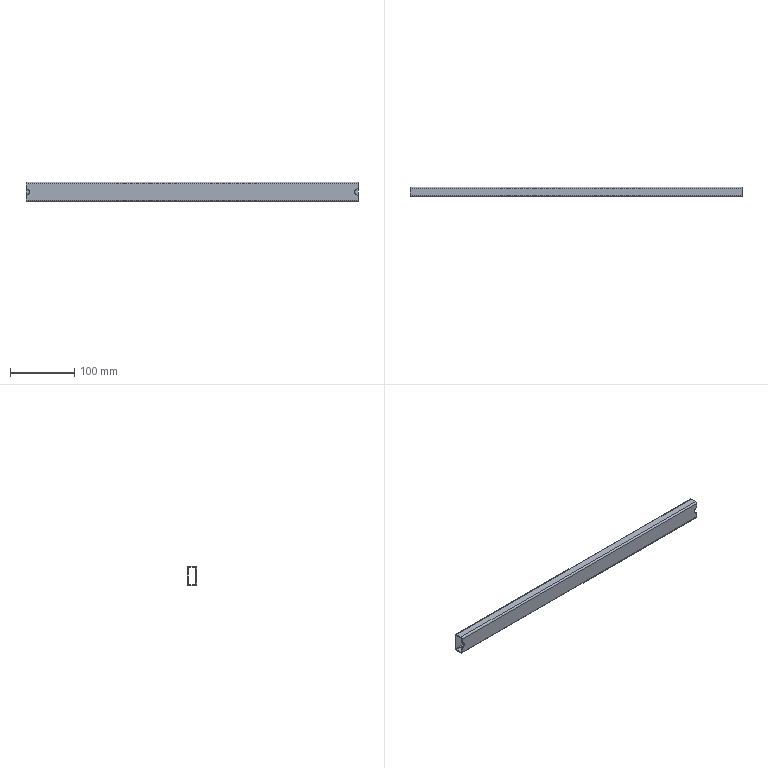Part | STEP file | 6150504 | 1 solid | 20 faces | box 515 x 15 x 30 mm | volume 62451 mm3 | plane 10 | cylinder 10 | commonest cylinder face diameters 2 x4 5 x4 10 x2
STEP:
#1=CARTESIAN_POINT('',(257.5,-7.5,-5.));
#2=VERTEX_POINT('',#1);
#3=CARTESIAN_POINT('',(257.5,-7.5,5.));
#4=VERTEX_POINT('',#3);
#5=CARTESIAN_POINT('',(257.5,-7.5,0.));
#6=DIRECTION('',(0.,1.,0.));
#7=DIRECTION('',(1.,0.,0.));
#8=AXIS2_PLACEMENT_3D('',#5,#6,#7);
#9=CIRCLE('',#8,5.);
#10=EDGE_CURVE('',#2,#4,#9,.T.);
#11=ORIENTED_EDGE('',*,*,#10,.T.);
#12=CARTESIAN_POINT('',(257.5,-7.5,12.5));
#13=VERTEX_POINT('',#12);
#14=CARTESIAN_POINT('',(257.5,-7.5,15.));
#15=DIRECTION('',(0.,0.,-1.));
#16=VECTOR('',#15,1000.);
#17=LINE('',#14,#16);
#18=EDGE_CURVE('',#13,#4,#17,.T.);
#19=ORIENTED_EDGE('',*,*,#18,.F.);
#20=CARTESIAN_POINT('',(-257.5,-7.5,12.5));
#21=VERTEX_POINT('',#20);
#22=CARTESIAN_POINT('',(-257.5,-7.5,12.5));
#23=DIRECTION('',(-1.,0.,0.));
#24=VECTOR('',#23,1000.);
#25=LINE('',#22,#24);
#26=EDGE_CURVE('',#13,#21,#25,.T.);
#27=ORIENTED_EDGE('',*,*,#26,.T.);
#28=CARTESIAN_POINT('',(-257.5,-7.5,5.));
#29=VERTEX_POINT('',#28);
#30=CARTESIAN_POINT('',(-257.5,-7.5,15.));
#31=DIRECTION('',(0.,0.,-1.));
#32=VECTOR('',#31,1000.);
#33=LINE('',#30,#32);
#34=EDGE_CURVE('',#21,#29,#33,.T.);
#35=ORIENTED_EDGE('',*,*,#34,.T.);
#36=CARTESIAN_POINT('',(-257.5,-7.5,-5.));
#37=VERTEX_POINT('',#36);
#38=CARTESIAN_POINT('',(-257.5,-7.5,0.));
#39=DIRECTION('',(0.,1.,0.));
#40=DIRECTION('',(-1.,0.,0.));
#41=AXIS2_PLACEMENT_3D('',#38,#39,#40);
#42=CIRCLE('',#41,5.);
#43=EDGE_CURVE('',#29,#37,#42,.T.);
#44=ORIENTED_EDGE('',*,*,#43,.T.);
#45=CARTESIAN_POINT('',(-257.5,-7.5,-12.5));
#46=VERTEX_POINT('',#45);
#47=CARTESIAN_POINT('',(-257.5,-7.5,15.));
#48=DIRECTION('',(0.,0.,-1.));
#49=VECTOR('',#48,1000.);
#50=LINE('',#47,#49);
#51=EDGE_CURVE('',#37,#46,#50,.T.);
#52=ORIENTED_EDGE('',*,*,#51,.T.);
#53=CARTESIAN_POINT('',(257.5,-7.5,-12.5));
#54=VERTEX_POINT('',#53);
#55=CARTESIAN_POINT('',(-257.5,-7.5,-12.5));
#56=DIRECTION('',(1.,0.,0.));
#57=VECTOR('',#56,1000.);
#58=LINE('',#55,#57);
#59=EDGE_CURVE('',#46,#54,#58,.T.);
#60=ORIENTED_EDGE('',*,*,#59,.T.);
#61=CARTESIAN_POINT('',(257.5,-7.5,15.));
#62=DIRECTION('',(0.,0.,-1.));
#63=VECTOR('',#62,1000.);
#64=LINE('',#61,#63);
#65=EDGE_CURVE('',#2,#54,#64,.T.);
#66=ORIENTED_EDGE('',*,*,#65,.F.);
#67=EDGE_LOOP('',(#11,#19,#27,#35,#44,#52,#60,#66));
#68=FACE_OUTER_BOUND('',#67,.T.);
#69=CARTESIAN_POINT('',(-257.5,-7.5,15.));
#70=DIRECTION('',(0.,1.,0.));
#71=DIRECTION('',(-1.,0.,0.));
#72=AXIS2_PLACEMENT_3D('',#69,#70,#71);
#73=PLANE('',#72);
#74=ADVANCED_FACE('',(#68),#73,.F.);
#75=CARTESIAN_POINT('',(257.5,-6.,12.5));
#76=VERTEX_POINT('',#75);
#77=CARTESIAN_POINT('',(257.5,-6.,5.));
#78=VERTEX_POINT('',#77);
#79=CARTESIAN_POINT('',(257.5,-6.,15.));
#80=DIRECTION('',(0.,0.,-1.));
#81=VECTOR('',#80,1000.);
#82=LINE('',#79,#81);
#83=EDGE_CURVE('',#76,#78,#82,.T.);
#84=ORIENTED_EDGE('',*,*,#83,.T.);
#85=CARTESIAN_POINT('',(257.5,-6.,-5.));
#86=VERTEX_POINT('',#85);
#87=CARTESIAN_POINT('',(257.5,-6.,0.));
#88=DIRECTION('',(0.,-1.,0.));
#89=DIRECTION('',(-1.,0.,0.));
#90=AXIS2_PLACEMENT_3D('',#87,#88,#89);
#91=CIRCLE('',#90,5.);
#92=EDGE_CURVE('',#78,#86,#91,.T.);
#93=ORIENTED_EDGE('',*,*,#92,.T.);
#94=CARTESIAN_POINT('',(257.5,-6.,-12.5));
#95=VERTEX_POINT('',#94);
#96=CARTESIAN_POINT('',(257.5,-6.,15.));
#97=DIRECTION('',(0.,0.,-1.));
#98=VECTOR('',#97,1000.);
#99=LINE('',#96,#98);
#100=EDGE_CURVE('',#86,#95,#99,.T.);
#101=ORIENTED_EDGE('',*,*,#100,.T.);
#102=CARTESIAN_POINT('',(-257.5,-6.,-12.5));
#103=VERTEX_POINT('',#102);
#104=CARTESIAN_POINT('',(-257.5,-6.,-12.5));
#105=DIRECTION('',(1.,0.,0.));
#106=VECTOR('',#105,1000.);
#107=LINE('',#104,#106);
#108=EDGE_CURVE('',#103,#95,#107,.T.);
#109=ORIENTED_EDGE('',*,*,#108,.F.);
#110=CARTESIAN_POINT('',(-257.5,-6.,-5.));
#111=VERTEX_POINT('',#110);
#112=CARTESIAN_POINT('',(-257.5,-6.,15.));
#113=DIRECTION('',(0.,0.,-1.));
#114=VECTOR('',#113,1000.);
#115=LINE('',#112,#114);
#116=EDGE_CURVE('',#111,#103,#115,.T.);
#117=ORIENTED_EDGE('',*,*,#116,.F.);
#118=CARTESIAN_POINT('',(-257.5,-6.,5.));
#119=VERTEX_POINT('',#118);
#120=CARTESIAN_POINT('',(-257.5,-6.,0.));
#121=DIRECTION('',(0.,-1.,0.));
#122=DIRECTION('',(-1.,0.,0.));
#123=AXIS2_PLACEMENT_3D('',#120,#121,#122);
#124=CIRCLE('',#123,5.);
#125=EDGE_CURVE('',#111,#119,#124,.T.);
#126=ORIENTED_EDGE('',*,*,#125,.T.);
#127=CARTESIAN_POINT('',(-257.5,-6.,12.5));
#128=VERTEX_POINT('',#127);
#129=CARTESIAN_POINT('',(-257.5,-6.,15.));
#130=DIRECTION('',(0.,0.,-1.));
#131=VECTOR('',#130,1000.);
#132=LINE('',#129,#131);
#133=EDGE_CURVE('',#128,#119,#132,.T.);
#134=ORIENTED_EDGE('',*,*,#133,.F.);
#135=CARTESIAN_POINT('',(-257.5,-6.,12.5));
#136=DIRECTION('',(-1.,0.,0.));
#137=VECTOR('',#136,1000.);
#138=LINE('',#135,#137);
#139=EDGE_CURVE('',#76,#128,#138,.T.);
#140=ORIENTED_EDGE('',*,*,#139,.F.);
#141=EDGE_LOOP('',(#84,#93,#101,#109,#117,#126,#134,#140));
#142=FACE_OUTER_BOUND('',#141,.T.);
#143=CARTESIAN_POINT('',(-257.5,-6.,15.));
#144=DIRECTION('',(0.,1.,0.));
#145=DIRECTION('',(-1.,0.,0.));
#146=AXIS2_PLACEMENT_3D('',#143,#144,#145);
#147=PLANE('',#146);
#148=ADVANCED_FACE('',(#142),#147,.T.);
#149=CARTESIAN_POINT('',(257.5,-3.,-5.));
#150=DIRECTION('',(0.,1.,0.));
#151=VECTOR('',#150,1000.);
#152=LINE('',#149,#151);
#153=EDGE_CURVE('',#2,#86,#152,.T.);
#154=ORIENTED_EDGE('',*,*,#153,.F.);
#155=ORIENTED_EDGE('',*,*,#65,.T.);
#156=CARTESIAN_POINT('',(257.5,-5.,-15.));
#157=VERTEX_POINT('',#156);
#158=CARTESIAN_POINT('',(257.5,-5.,-12.5));
#159=DIRECTION('',(1.,0.,0.));
#160=DIRECTION('',(0.,0.,1.));
#161=AXIS2_PLACEMENT_3D('',#158,#159,#160);
#162=CIRCLE('',#161,2.5);
#163=EDGE_CURVE('',#54,#157,#162,.T.);
#164=ORIENTED_EDGE('',*,*,#163,.T.);
#165=CARTESIAN_POINT('',(257.5,5.,-15.));
#166=VERTEX_POINT('',#165);
#167=CARTESIAN_POINT('',(257.5,7.5,-15.));
#168=DIRECTION('',(0.,1.,0.));
#169=VECTOR('',#168,1000.);
#170=LINE('',#167,#169);
#171=EDGE_CURVE('',#157,#166,#170,.T.);
#172=ORIENTED_EDGE('',*,*,#171,.T.);
#173=CARTESIAN_POINT('',(257.5,7.5,-12.5));
#174=VERTEX_POINT('',#173);
#175=CARTESIAN_POINT('',(257.5,5.,-12.5));
#176=DIRECTION('',(1.,0.,0.));
#177=DIRECTION('',(0.,0.,1.));
#178=AXIS2_PLACEMENT_3D('',#175,#176,#177);
#179=CIRCLE('',#178,2.5);
#180=EDGE_CURVE('',#166,#174,#179,.T.);
#181=ORIENTED_EDGE('',*,*,#180,.T.);
#182=CARTESIAN_POINT('',(257.5,7.5,12.5));
#183=VERTEX_POINT('',#182);
#184=CARTESIAN_POINT('',(257.5,7.5,15.));
#185=DIRECTION('',(0.,0.,-1.));
#186=VECTOR('',#185,1000.);
#187=LINE('',#184,#186);
#188=EDGE_CURVE('',#183,#174,#187,.T.);
#189=ORIENTED_EDGE('',*,*,#188,.F.);
#190=CARTESIAN_POINT('',(257.5,5.,15.));
#191=VERTEX_POINT('',#190);
#192=CARTESIAN_POINT('',(257.5,5.,12.5));
#193=DIRECTION('',(1.,0.,0.));
#194=DIRECTION('',(0.,0.,1.));
#195=AXIS2_PLACEMENT_3D('',#192,#193,#194);
#196=CIRCLE('',#195,2.5);
#197=EDGE_CURVE('',#183,#191,#196,.T.);
#198=ORIENTED_EDGE('',*,*,#197,.T.);
#199=CARTESIAN_POINT('',(257.5,-5.,15.));
#200=VERTEX_POINT('',#199);
#201=CARTESIAN_POINT('',(257.5,7.5,15.));
#202=DIRECTION('',(0.,1.,0.));
#203=VECTOR('',#202,1000.);
#204=LINE('',#201,#203);
#205=EDGE_CURVE('',#200,#191,#204,.T.);
#206=ORIENTED_EDGE('',*,*,#205,.F.);
#207=CARTESIAN_POINT('',(257.5,-5.,12.5));
#208=DIRECTION('',(1.,0.,0.));
#209=DIRECTION('',(0.,0.,1.));
#210=AXIS2_PLACEMENT_3D('',#207,#208,#209);
#211=CIRCLE('',#210,2.5);
#212=EDGE_CURVE('',#200,#13,#211,.T.);
#213=ORIENTED_EDGE('',*,*,#212,.T.);
#214=ORIENTED_EDGE('',*,*,#18,.T.);
#215=CARTESIAN_POINT('',(257.5,-3.,5.));
#216=DIRECTION('',(0.,-1.,0.));
#217=VECTOR('',#216,1000.);
#218=LINE('',#215,#217);
#219=EDGE_CURVE('',#78,#4,#218,.T.);
#220=ORIENTED_EDGE('',*,*,#219,.F.);
#221=ORIENTED_EDGE('',*,*,#83,.F.);
#222=CARTESIAN_POINT('',(257.5,-5.,13.5));
#223=VERTEX_POINT('',#222);
#224=CARTESIAN_POINT('',(257.5,-5.,12.5));
#225=DIRECTION('',(1.,0.,0.));
#226=DIRECTION('',(0.,0.,1.));
#227=AXIS2_PLACEMENT_3D('',#224,#225,#226);
#228=CIRCLE('',#227,1.);
#229=EDGE_CURVE('',#223,#76,#228,.T.);
#230=ORIENTED_EDGE('',*,*,#229,.F.);
#231=CARTESIAN_POINT('',(257.5,5.,13.5));
#232=VERTEX_POINT('',#231);
#233=CARTESIAN_POINT('',(257.5,7.5,13.5));
#234=DIRECTION('',(0.,1.,0.));
#235=VECTOR('',#234,1000.);
#236=LINE('',#233,#235);
#237=EDGE_CURVE('',#223,#232,#236,.T.);
#238=ORIENTED_EDGE('',*,*,#237,.T.);
#239=CARTESIAN_POINT('',(257.5,6.,12.5));
#240=VERTEX_POINT('',#239);
#241=CARTESIAN_POINT('',(257.5,5.,12.5));
#242=DIRECTION('',(1.,0.,0.));
#243=DIRECTION('',(0.,0.,1.));
#244=AXIS2_PLACEMENT_3D('',#241,#242,#243);
#245=CIRCLE('',#244,1.);
#246=EDGE_CURVE('',#240,#232,#245,.T.);
#247=ORIENTED_EDGE('',*,*,#246,.F.);
#248=CARTESIAN_POINT('',(257.5,6.,-12.5));
#249=VERTEX_POINT('',#248);
#250=CARTESIAN_POINT('',(257.5,6.,15.));
#251=DIRECTION('',(0.,0.,-1.));
#252=VECTOR('',#251,1000.);
#253=LINE('',#250,#252);
#254=EDGE_CURVE('',#240,#249,#253,.T.);
#255=ORIENTED_EDGE('',*,*,#254,.T.);
#256=CARTESIAN_POINT('',(257.5,5.,-13.5));
#257=VERTEX_POINT('',#256);
#258=CARTESIAN_POINT('',(257.5,5.,-12.5));
#259=DIRECTION('',(1.,0.,0.));
#260=DIRECTION('',(0.,0.,1.));
#261=AXIS2_PLACEMENT_3D('',#258,#259,#260);
#262=CIRCLE('',#261,1.);
#263=EDGE_CURVE('',#257,#249,#262,.T.);
#264=ORIENTED_EDGE('',*,*,#263,.F.);
#265=CARTESIAN_POINT('',(257.5,-5.,-13.5));
#266=VERTEX_POINT('',#265);
#267=CARTESIAN_POINT('',(257.5,7.5,-13.5));
#268=DIRECTION('',(0.,1.,0.));
#269=VECTOR('',#268,1000.);
#270=LINE('',#267,#269);
#271=EDGE_CURVE('',#266,#257,#270,.T.);
#272=ORIENTED_EDGE('',*,*,#271,.F.);
#273=CARTESIAN_POINT('',(257.5,-5.,-12.5));
#274=DIRECTION('',(1.,0.,0.));
#275=DIRECTION('',(0.,0.,1.));
#276=AXIS2_PLACEMENT_3D('',#273,#274,#275);
#277=CIRCLE('',#276,1.);
#278=EDGE_CURVE('',#95,#266,#277,.T.);
#279=ORIENTED_EDGE('',*,*,#278,.F.);
#280=ORIENTED_EDGE('',*,*,#100,.F.);
#281=EDGE_LOOP('',(#154,#155,#164,#172,#181,#189,#198,#206,#213,#214,#220,#221,#230,#238,#247,#255,#264,#272,#279,#280));
#282=FACE_OUTER_BOUND('',#281,.T.);
#283=CARTESIAN_POINT('',(257.5,7.5,15.));
#284=DIRECTION('',(-1.,0.,0.));
#285=DIRECTION('',(0.,0.,1.));
#286=AXIS2_PLACEMENT_3D('',#283,#284,#285);
#287=PLANE('',#286);
#288=ADVANCED_FACE('',(#282),#287,.F.);
#289=CARTESIAN_POINT('',(-257.5,-3.,5.));
#290=DIRECTION('',(0.,1.,0.));
#291=VECTOR('',#290,1000.);
#292=LINE('',#289,#291);
#293=EDGE_CURVE('',#29,#119,#292,.T.);
#294=ORIENTED_EDGE('',*,*,#293,.F.);
#295=ORIENTED_EDGE('',*,*,#34,.F.);
#296=CARTESIAN_POINT('',(-257.5,-5.,15.));
#297=VERTEX_POINT('',#296);
#298=CARTESIAN_POINT('',(-257.5,-5.,12.5));
#299=DIRECTION('',(-1.,0.,0.));
#300=DIRECTION('',(0.,0.,-1.));
#301=AXIS2_PLACEMENT_3D('',#298,#299,#300);
#302=CIRCLE('',#301,2.5);
#303=EDGE_CURVE('',#21,#297,#302,.T.);
#304=ORIENTED_EDGE('',*,*,#303,.T.);
#305=CARTESIAN_POINT('',(-257.5,5.,15.));
#306=VERTEX_POINT('',#305);
#307=CARTESIAN_POINT('',(-257.5,7.5,15.));
#308=DIRECTION('',(0.,-1.,0.));
#309=VECTOR('',#308,1000.);
#310=LINE('',#307,#309);
#311=EDGE_CURVE('',#306,#297,#310,.T.);
#312=ORIENTED_EDGE('',*,*,#311,.F.);
#313=CARTESIAN_POINT('',(-257.5,7.5,12.5));
#314=VERTEX_POINT('',#313);
#315=CARTESIAN_POINT('',(-257.5,5.,12.5));
#316=DIRECTION('',(-1.,0.,0.));
#317=DIRECTION('',(0.,0.,-1.));
#318=AXIS2_PLACEMENT_3D('',#315,#316,#317);
#319=CIRCLE('',#318,2.5);
#320=EDGE_CURVE('',#306,#314,#319,.T.);
#321=ORIENTED_EDGE('',*,*,#320,.T.);
#322=CARTESIAN_POINT('',(-257.5,7.5,-12.5));
#323=VERTEX_POINT('',#322);
#324=CARTESIAN_POINT('',(-257.5,7.5,15.));
#325=DIRECTION('',(0.,0.,-1.));
#326=VECTOR('',#325,1000.);
#327=LINE('',#324,#326);
#328=EDGE_CURVE('',#314,#323,#327,.T.);
#329=ORIENTED_EDGE('',*,*,#328,.T.);
#330=CARTESIAN_POINT('',(-257.5,5.,-15.));
#331=VERTEX_POINT('',#330);
#332=CARTESIAN_POINT('',(-257.5,5.,-12.5));
#333=DIRECTION('',(-1.,0.,0.));
#334=DIRECTION('',(0.,0.,-1.));
#335=AXIS2_PLACEMENT_3D('',#332,#333,#334);
#336=CIRCLE('',#335,2.5);
#337=EDGE_CURVE('',#323,#331,#336,.T.);
#338=ORIENTED_EDGE('',*,*,#337,.T.);
#339=CARTESIAN_POINT('',(-257.5,-5.,-15.));
#340=VERTEX_POINT('',#339);
#341=CARTESIAN_POINT('',(-257.5,7.5,-15.));
#342=DIRECTION('',(0.,-1.,0.));
#343=VECTOR('',#342,1000.);
#344=LINE('',#341,#343);
#345=EDGE_CURVE('',#331,#340,#344,.T.);
#346=ORIENTED_EDGE('',*,*,#345,.T.);
#347=CARTESIAN_POINT('',(-257.5,-5.,-12.5));
#348=DIRECTION('',(-1.,0.,0.));
#349=DIRECTION('',(0.,0.,-1.));
#350=AXIS2_PLACEMENT_3D('',#347,#348,#349);
#351=CIRCLE('',#350,2.5);
#352=EDGE_CURVE('',#340,#46,#351,.T.);
#353=ORIENTED_EDGE('',*,*,#352,.T.);
#354=ORIENTED_EDGE('',*,*,#51,.F.);
#355=CARTESIAN_POINT('',(-257.5,-3.,-5.));
#356=DIRECTION('',(0.,-1.,0.));
#357=VECTOR('',#356,1000.);
#358=LINE('',#355,#357);
#359=EDGE_CURVE('',#111,#37,#358,.T.);
#360=ORIENTED_EDGE('',*,*,#359,.F.);
#361=ORIENTED_EDGE('',*,*,#116,.T.);
#362=CARTESIAN_POINT('',(-257.5,-5.,-13.5));
#363=VERTEX_POINT('',#362);
#364=CARTESIAN_POINT('',(-257.5,-5.,-12.5));
#365=DIRECTION('',(-1.,0.,0.));
#366=DIRECTION('',(0.,0.,-1.));
#367=AXIS2_PLACEMENT_3D('',#364,#365,#366);
#368=CIRCLE('',#367,1.);
#369=EDGE_CURVE('',#363,#103,#368,.T.);
#370=ORIENTED_EDGE('',*,*,#369,.F.);
#371=CARTESIAN_POINT('',(-257.5,5.,-13.5));
#372=VERTEX_POINT('',#371);
#373=CARTESIAN_POINT('',(-257.5,7.5,-13.5));
#374=DIRECTION('',(0.,-1.,0.));
#375=VECTOR('',#374,1000.);
#376=LINE('',#373,#375);
#377=EDGE_CURVE('',#372,#363,#376,.T.);
#378=ORIENTED_EDGE('',*,*,#377,.F.);
#379=CARTESIAN_POINT('',(-257.5,6.,-12.5));
#380=VERTEX_POINT('',#379);
#381=CARTESIAN_POINT('',(-257.5,5.,-12.5));
#382=DIRECTION('',(-1.,0.,0.));
#383=DIRECTION('',(0.,0.,-1.));
#384=AXIS2_PLACEMENT_3D('',#381,#382,#383);
#385=CIRCLE('',#384,1.);
#386=EDGE_CURVE('',#380,#372,#385,.T.);
#387=ORIENTED_EDGE('',*,*,#386,.F.);
#388=CARTESIAN_POINT('',(-257.5,6.,12.5));
#389=VERTEX_POINT('',#388);
#390=CARTESIAN_POINT('',(-257.5,6.,15.));
#391=DIRECTION('',(0.,0.,-1.));
#392=VECTOR('',#391,1000.);
#393=LINE('',#390,#392);
#394=EDGE_CURVE('',#389,#380,#393,.T.);
#395=ORIENTED_EDGE('',*,*,#394,.F.);
#396=CARTESIAN_POINT('',(-257.5,5.,13.5));
#397=VERTEX_POINT('',#396);
#398=CARTESIAN_POINT('',(-257.5,5.,12.5));
#399=DIRECTION('',(-1.,0.,0.));
#400=DIRECTION('',(0.,0.,-1.));
#401=AXIS2_PLACEMENT_3D('',#398,#399,#400);
#402=CIRCLE('',#401,1.);
#403=EDGE_CURVE('',#397,#389,#402,.T.);
#404=ORIENTED_EDGE('',*,*,#403,.F.);
#405=CARTESIAN_POINT('',(-257.5,-5.,13.5));
#406=VERTEX_POINT('',#405);
#407=CARTESIAN_POINT('',(-257.5,7.5,13.5));
#408=DIRECTION('',(0.,-1.,0.));
#409=VECTOR('',#408,1000.);
#410=LINE('',#407,#409);
#411=EDGE_CURVE('',#397,#406,#410,.T.);
#412=ORIENTED_EDGE('',*,*,#411,.T.);
#413=CARTESIAN_POINT('',(-257.5,-5.,12.5));
#414=DIRECTION('',(-1.,0.,0.));
#415=DIRECTION('',(0.,0.,-1.));
#416=AXIS2_PLACEMENT_3D('',#413,#414,#415);
#417=CIRCLE('',#416,1.);
#418=EDGE_CURVE('',#128,#406,#417,.T.);
#419=ORIENTED_EDGE('',*,*,#418,.F.);
#420=ORIENTED_EDGE('',*,*,#133,.T.);
#421=EDGE_LOOP('',(#294,#295,#304,#312,#321,#329,#338,#346,#353,#354,#360,#361,#370,#378,#387,#395,#404,#412,#419,#420));
#422=FACE_OUTER_BOUND('',#421,.T.);
#423=CARTESIAN_POINT('',(-257.5,7.5,15.));
#424=DIRECTION('',(1.,0.,0.));
#425=DIRECTION('',(0.,0.,-1.));
#426=AXIS2_PLACEMENT_3D('',#423,#424,#425);
#427=PLANE('',#426);
#428=ADVANCED_FACE('',(#422),#427,.F.);
#429=ORIENTED_EDGE('',*,*,#188,.T.);
#430=CARTESIAN_POINT('',(-257.5,7.5,-12.5));
#431=DIRECTION('',(-1.,0.,0.));
#432=VECTOR('',#431,1000.);
#433=LINE('',#430,#432);
#434=EDGE_CURVE('',#174,#323,#433,.T.);
#435=ORIENTED_EDGE('',*,*,#434,.T.);
#436=ORIENTED_EDGE('',*,*,#328,.F.);
#437=CARTESIAN_POINT('',(257.5,7.5,12.5));
#438=DIRECTION('',(1.,0.,0.));
#439=VECTOR('',#438,1000.);
#440=LINE('',#437,#439);
#441=EDGE_CURVE('',#314,#183,#440,.T.);
#442=ORIENTED_EDGE('',*,*,#441,.T.);
#443=EDGE_LOOP('',(#429,#435,#436,#442));
#444=FACE_OUTER_BOUND('',#443,.T.);
#445=CARTESIAN_POINT('',(-257.5,7.5,15.));
#446=DIRECTION('',(0.,-1.,0.));
#447=DIRECTION('',(0.,0.,-1.));
#448=AXIS2_PLACEMENT_3D('',#445,#446,#447);
#449=PLANE('',#448);
#450=ADVANCED_FACE('',(#444),#449,.F.);
#451=ORIENTED_EDGE('',*,*,#311,.T.);
#452=CARTESIAN_POINT('',(257.5,-5.,15.));
#453=DIRECTION('',(1.,0.,0.));
#454=VECTOR('',#453,1000.);
#455=LINE('',#452,#454);
#456=EDGE_CURVE('',#297,#200,#455,.T.);
#457=ORIENTED_EDGE('',*,*,#456,.T.);
#458=ORIENTED_EDGE('',*,*,#205,.T.);
#459=CARTESIAN_POINT('',(-257.5,5.,15.));
#460=DIRECTION('',(-1.,0.,0.));
#461=VECTOR('',#460,1000.);
#462=LINE('',#459,#461);
#463=EDGE_CURVE('',#191,#306,#462,.T.);
#464=ORIENTED_EDGE('',*,*,#463,.T.);
#465=EDGE_LOOP('',(#451,#457,#458,#464));
#466=FACE_OUTER_BOUND('',#465,.T.);
#467=CARTESIAN_POINT('',(-257.5,7.5,15.));
#468=DIRECTION('',(0.,0.,1.));
#469=DIRECTION('',(1.,0.,0.));
#470=AXIS2_PLACEMENT_3D('',#467,#468,#469);
#471=PLANE('',#470);
#472=ADVANCED_FACE('',(#466),#471,.T.);
#473=ORIENTED_EDGE('',*,*,#345,.F.);
#474=CARTESIAN_POINT('',(-257.5,5.,-15.));
#475=DIRECTION('',(1.,0.,0.));
#476=VECTOR('',#475,1000.);
#477=LINE('',#474,#476);
#478=EDGE_CURVE('',#331,#166,#477,.T.);
#479=ORIENTED_EDGE('',*,*,#478,.T.);
#480=ORIENTED_EDGE('',*,*,#171,.F.);
#481=CARTESIAN_POINT('',(-257.5,-5.,-15.));
#482=DIRECTION('',(-1.,0.,0.));
#483=VECTOR('',#482,1000.);
#484=LINE('',#481,#483);
#485=EDGE_CURVE('',#157,#340,#484,.T.);
#486=ORIENTED_EDGE('',*,*,#485,.T.);
#487=EDGE_LOOP('',(#473,#479,#480,#486));
#488=FACE_OUTER_BOUND('',#487,.T.);
#489=CARTESIAN_POINT('',(-257.5,7.5,-15.));
#490=DIRECTION('',(0.,0.,1.));
#491=DIRECTION('',(1.,0.,0.));
#492=AXIS2_PLACEMENT_3D('',#489,#490,#491);
#493=PLANE('',#492);
#494=ADVANCED_FACE('',(#488),#493,.F.);
#495=ORIENTED_EDGE('',*,*,#303,.F.);
#496=ORIENTED_EDGE('',*,*,#26,.F.);
#497=ORIENTED_EDGE('',*,*,#212,.F.);
#498=ORIENTED_EDGE('',*,*,#456,.F.);
#499=EDGE_LOOP('',(#495,#496,#497,#498));
#500=FACE_OUTER_BOUND('',#499,.T.);
#501=CARTESIAN_POINT('',(-257.5,-5.,12.5));
#502=DIRECTION('',(-1.,0.,0.));
#503=DIRECTION('',(0.,-1.,0.));
#504=AXIS2_PLACEMENT_3D('',#501,#502,#503);
#505=CYLINDRICAL_SURFACE('',#504,2.5);
#506=ADVANCED_FACE('',(#500),#505,.T.);
#507=ORIENTED_EDGE('',*,*,#180,.F.);
#508=ORIENTED_EDGE('',*,*,#478,.F.);
#509=ORIENTED_EDGE('',*,*,#337,.F.);
#510=ORIENTED_EDGE('',*,*,#434,.F.);
#511=EDGE_LOOP('',(#507,#508,#509,#510));
#512=FACE_OUTER_BOUND('',#511,.T.);
#513=CARTESIAN_POINT('',(-257.5,5.,-12.5));
#514=DIRECTION('',(-1.,0.,0.));
#515=DIRECTION('',(0.,0.,1.));
#516=AXIS2_PLACEMENT_3D('',#513,#514,#515);
#517=CYLINDRICAL_SURFACE('',#516,2.5);
#518=ADVANCED_FACE('',(#512),#517,.T.);
#519=ORIENTED_EDGE('',*,*,#352,.F.);
#520=ORIENTED_EDGE('',*,*,#485,.F.);
#521=ORIENTED_EDGE('',*,*,#163,.F.);
#522=ORIENTED_EDGE('',*,*,#59,.F.);
#523=EDGE_LOOP('',(#519,#520,#521,#522));
#524=FACE_OUTER_BOUND('',#523,.T.);
#525=CARTESIAN_POINT('',(-257.5,-5.,-12.5));
#526=DIRECTION('',(1.,0.,0.));
#527=DIRECTION('',(0.,1.,0.));
#528=AXIS2_PLACEMENT_3D('',#525,#526,#527);
#529=CYLINDRICAL_SURFACE('',#528,2.5);
#530=ADVANCED_FACE('',(#524),#529,.T.);
#531=ORIENTED_EDGE('',*,*,#197,.F.);
#532=ORIENTED_EDGE('',*,*,#441,.F.);
#533=ORIENTED_EDGE('',*,*,#320,.F.);
#534=ORIENTED_EDGE('',*,*,#463,.F.);
#535=EDGE_LOOP('',(#531,#532,#533,#534));
#536=FACE_OUTER_BOUND('',#535,.T.);
#537=CARTESIAN_POINT('',(-257.5,5.,12.5));
#538=DIRECTION('',(1.,0.,0.));
#539=DIRECTION('',(0.,0.,-1.));
#540=AXIS2_PLACEMENT_3D('',#537,#538,#539);
#541=CYLINDRICAL_SURFACE('',#540,2.5);
#542=ADVANCED_FACE('',(#536),#541,.T.);
#543=ORIENTED_EDGE('',*,*,#254,.F.);
#544=CARTESIAN_POINT('',(-257.5,6.,12.5));
#545=DIRECTION('',(1.,0.,0.));
#546=VECTOR('',#545,1000.);
#547=LINE('',#544,#546);
#548=EDGE_CURVE('',#389,#240,#547,.T.);
#549=ORIENTED_EDGE('',*,*,#548,.F.);
#550=ORIENTED_EDGE('',*,*,#394,.T.);
#551=CARTESIAN_POINT('',(-257.5,6.,-12.5));
#552=DIRECTION('',(-1.,0.,0.));
#553=VECTOR('',#552,1000.);
#554=LINE('',#551,#553);
#555=EDGE_CURVE('',#249,#380,#554,.T.);
#556=ORIENTED_EDGE('',*,*,#555,.F.);
#557=EDGE_LOOP('',(#543,#549,#550,#556));
#558=FACE_OUTER_BOUND('',#557,.T.);
#559=CARTESIAN_POINT('',(-257.5,6.,15.));
#560=DIRECTION('',(0.,-1.,0.));
#561=DIRECTION('',(0.,0.,-1.));
#562=AXIS2_PLACEMENT_3D('',#559,#560,#561);
#563=PLANE('',#562);
#564=ADVANCED_FACE('',(#558),#563,.T.);
#565=ORIENTED_EDGE('',*,*,#411,.F.);
#566=CARTESIAN_POINT('',(-257.5,5.,13.5));
#567=DIRECTION('',(-1.,0.,0.));
#568=VECTOR('',#567,1000.);
#569=LINE('',#566,#568);
#570=EDGE_CURVE('',#232,#397,#569,.T.);
#571=ORIENTED_EDGE('',*,*,#570,.F.);
#572=ORIENTED_EDGE('',*,*,#237,.F.);
#573=CARTESIAN_POINT('',(-257.5,-5.,13.5));
#574=DIRECTION('',(1.,0.,0.));
#575=VECTOR('',#574,1000.);
#576=LINE('',#573,#575);
#577=EDGE_CURVE('',#406,#223,#576,.T.);
#578=ORIENTED_EDGE('',*,*,#577,.F.);
#579=EDGE_LOOP('',(#565,#571,#572,#578));
#580=FACE_OUTER_BOUND('',#579,.T.);
#581=CARTESIAN_POINT('',(-257.5,7.5,13.5));
#582=DIRECTION('',(0.,0.,1.));
#583=DIRECTION('',(1.,0.,0.));
#584=AXIS2_PLACEMENT_3D('',#581,#582,#583);
#585=PLANE('',#584);
#586=ADVANCED_FACE('',(#580),#585,.F.);
#587=ORIENTED_EDGE('',*,*,#377,.T.);
#588=CARTESIAN_POINT('',(-257.5,-5.,-13.5));
#589=DIRECTION('',(-1.,0.,0.));
#590=VECTOR('',#589,1000.);
#591=LINE('',#588,#590);
#592=EDGE_CURVE('',#266,#363,#591,.T.);
#593=ORIENTED_EDGE('',*,*,#592,.F.);
#594=ORIENTED_EDGE('',*,*,#271,.T.);
#595=CARTESIAN_POINT('',(-257.5,5.,-13.5));
#596=DIRECTION('',(1.,0.,0.));
#597=VECTOR('',#596,1000.);
#598=LINE('',#595,#597);
#599=EDGE_CURVE('',#372,#257,#598,.T.);
#600=ORIENTED_EDGE('',*,*,#599,.F.);
#601=EDGE_LOOP('',(#587,#593,#594,#600));
#602=FACE_OUTER_BOUND('',#601,.T.);
#603=CARTESIAN_POINT('',(-257.5,7.5,-13.5));
#604=DIRECTION('',(0.,0.,1.));
#605=DIRECTION('',(1.,0.,0.));
#606=AXIS2_PLACEMENT_3D('',#603,#604,#605);
#607=PLANE('',#606);
#608=ADVANCED_FACE('',(#602),#607,.T.);
#609=ORIENTED_EDGE('',*,*,#418,.T.);
#610=ORIENTED_EDGE('',*,*,#577,.T.);
#611=ORIENTED_EDGE('',*,*,#229,.T.);
#612=ORIENTED_EDGE('',*,*,#139,.T.);
#613=EDGE_LOOP('',(#609,#610,#611,#612));
#614=FACE_OUTER_BOUND('',#613,.T.);
#615=CARTESIAN_POINT('',(-257.5,-5.,12.5));
#616=DIRECTION('',(-1.,0.,0.));
#617=DIRECTION('',(0.,-1.,0.));
#618=AXIS2_PLACEMENT_3D('',#615,#616,#617);
#619=CYLINDRICAL_SURFACE('',#618,1.);
#620=ADVANCED_FACE('',(#614),#619,.F.);
#621=ORIENTED_EDGE('',*,*,#263,.T.);
#622=ORIENTED_EDGE('',*,*,#555,.T.);
#623=ORIENTED_EDGE('',*,*,#386,.T.);
#624=ORIENTED_EDGE('',*,*,#599,.T.);
#625=EDGE_LOOP('',(#621,#622,#623,#624));
#626=FACE_OUTER_BOUND('',#625,.T.);
#627=CARTESIAN_POINT('',(-257.5,5.,-12.5));
#628=DIRECTION('',(-1.,0.,0.));
#629=DIRECTION('',(0.,0.,1.));
#630=AXIS2_PLACEMENT_3D('',#627,#628,#629);
#631=CYLINDRICAL_SURFACE('',#630,1.);
#632=ADVANCED_FACE('',(#626),#631,.F.);
#633=ORIENTED_EDGE('',*,*,#369,.T.);
#634=ORIENTED_EDGE('',*,*,#108,.T.);
#635=ORIENTED_EDGE('',*,*,#278,.T.);
#636=ORIENTED_EDGE('',*,*,#592,.T.);
#637=EDGE_LOOP('',(#633,#634,#635,#636));
#638=FACE_OUTER_BOUND('',#637,.T.);
#639=CARTESIAN_POINT('',(-257.5,-5.,-12.5));
#640=DIRECTION('',(1.,0.,0.));
#641=DIRECTION('',(0.,1.,0.));
#642=AXIS2_PLACEMENT_3D('',#639,#640,#641);
#643=CYLINDRICAL_SURFACE('',#642,1.);
#644=ADVANCED_FACE('',(#638),#643,.F.);
#645=ORIENTED_EDGE('',*,*,#246,.T.);
#646=ORIENTED_EDGE('',*,*,#570,.T.);
#647=ORIENTED_EDGE('',*,*,#403,.T.);
#648=ORIENTED_EDGE('',*,*,#548,.T.);
#649=EDGE_LOOP('',(#645,#646,#647,#648));
#650=FACE_OUTER_BOUND('',#649,.T.);
#651=CARTESIAN_POINT('',(-257.5,5.,12.5));
#652=DIRECTION('',(1.,0.,0.));
#653=DIRECTION('',(0.,0.,-1.));
#654=AXIS2_PLACEMENT_3D('',#651,#652,#653);
#655=CYLINDRICAL_SURFACE('',#654,1.);
#656=ADVANCED_FACE('',(#650),#655,.F.);
#657=ORIENTED_EDGE('',*,*,#293,.T.);
#658=ORIENTED_EDGE('',*,*,#125,.F.);
#659=ORIENTED_EDGE('',*,*,#359,.T.);
#660=ORIENTED_EDGE('',*,*,#43,.F.);
#661=EDGE_LOOP('',(#657,#658,#659,#660));
#662=FACE_OUTER_BOUND('',#661,.T.);
#663=CARTESIAN_POINT('',(-257.5,-3.,0.));
#664=DIRECTION('',(0.,-1.,0.));
#665=DIRECTION('',(1.,0.,0.));
#666=AXIS2_PLACEMENT_3D('',#663,#664,#665);
#667=CYLINDRICAL_SURFACE('',#666,5.);
#668=ADVANCED_FACE('',(#662),#667,.F.);
#669=ORIENTED_EDGE('',*,*,#153,.T.);
#670=ORIENTED_EDGE('',*,*,#92,.F.);
#671=ORIENTED_EDGE('',*,*,#219,.T.);
#672=ORIENTED_EDGE('',*,*,#10,.F.);
#673=EDGE_LOOP('',(#669,#670,#671,#672));
#674=FACE_OUTER_BOUND('',#673,.T.);
#675=CARTESIAN_POINT('',(257.5,-3.,0.));
#676=DIRECTION('',(0.,-1.,0.));
#677=DIRECTION('',(1.,0.,0.));
#678=AXIS2_PLACEMENT_3D('',#675,#676,#677);
#679=CYLINDRICAL_SURFACE('',#678,5.);
#680=ADVANCED_FACE('',(#674),#679,.F.);
#681=CLOSED_SHELL('',(#74,#148,#288,#428,#450,#472,#494,#506,#518,#530,#542,#564,#586,#608,#620,#632,#644,#656,#668,#680));
#682=MANIFOLD_SOLID_BREP('',#681);
#683=CARTESIAN_POINT('',(0.,0.,0.));
#684=DIRECTION('',(0.,0.,1.));
#685=DIRECTION('',(1.,0.,0.));
#686=AXIS2_PLACEMENT_3D('',#683,#684,#685);
#687=(LENGTH_UNIT()NAMED_UNIT(*)SI_UNIT(.MILLI.,.METRE.));
#688=UNCERTAINTY_MEASURE_WITH_UNIT(LENGTH_MEASURE(0.00001),#687,'','');
#689=(NAMED_UNIT(*)PLANE_ANGLE_UNIT()SI_UNIT($,.RADIAN.));
#690=(NAMED_UNIT(*)SI_UNIT($,.STERADIAN.)SOLID_ANGLE_UNIT());
#691=(GEOMETRIC_REPRESENTATION_CONTEXT(3)GLOBAL_UNCERTAINTY_ASSIGNED_CONTEXT((#688))GLOBAL_UNIT_ASSIGNED_CONTEXT((#687,#689,#690))REPRESENTATION_CONTEXT('',''));
#692=ADVANCED_BREP_SHAPE_REPRESENTATION('',(#682,#686),#691);